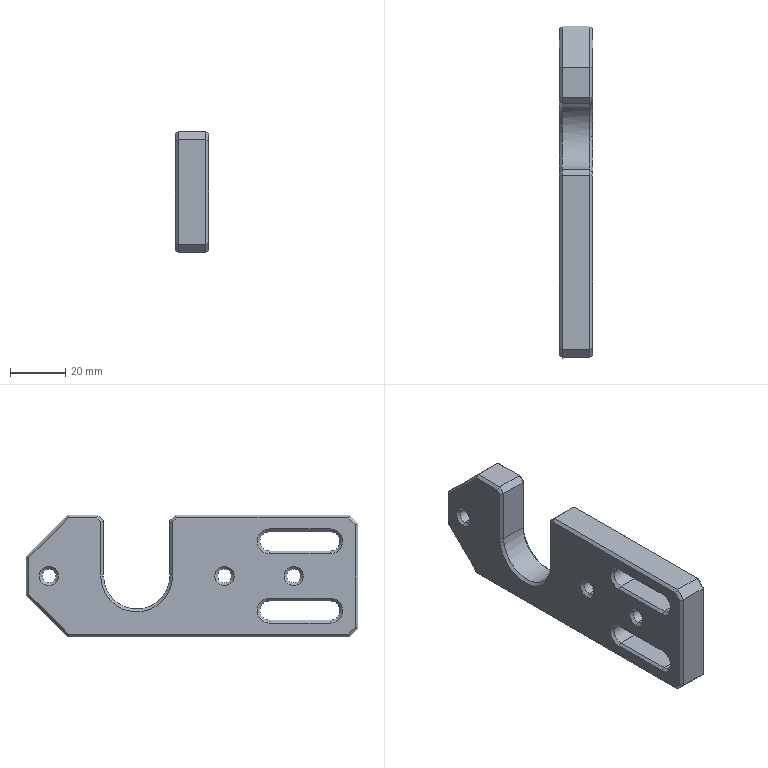Part | SolidWorks | features BaseBody 1 | 1 solid | 87 faces | box 12 x 120 x 44 mm | volume 45578 mm3 | plane 53 | cone 23 | cylinder 11 | commonest cylinder face diameters 5 x6 7 x4 24 x1